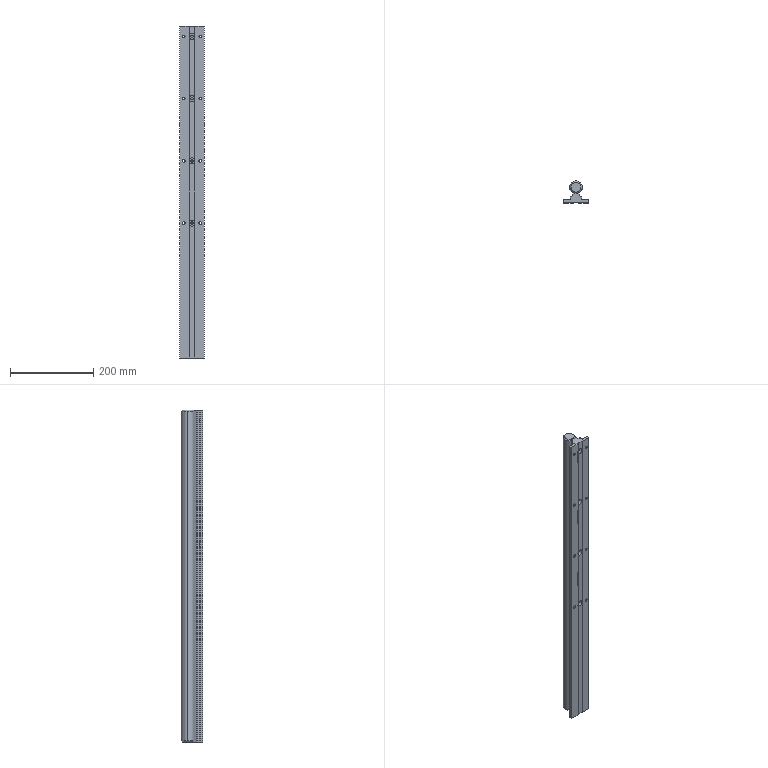Part | SolidWorks | features RevCut 2, Chamfer 1, CurvePattern 1, Extrusion 1, ICE 1, MirrorPattern 1 | 1 solid | 82 faces | box 60 x 52 x 800 mm | volume 1150861 mm3 | cylinder 47 | plane 31 | cone 4 | commonest cylinder face diameters 6.6 x16 1.4 x10 5.6 x8 14 x8 30 x5